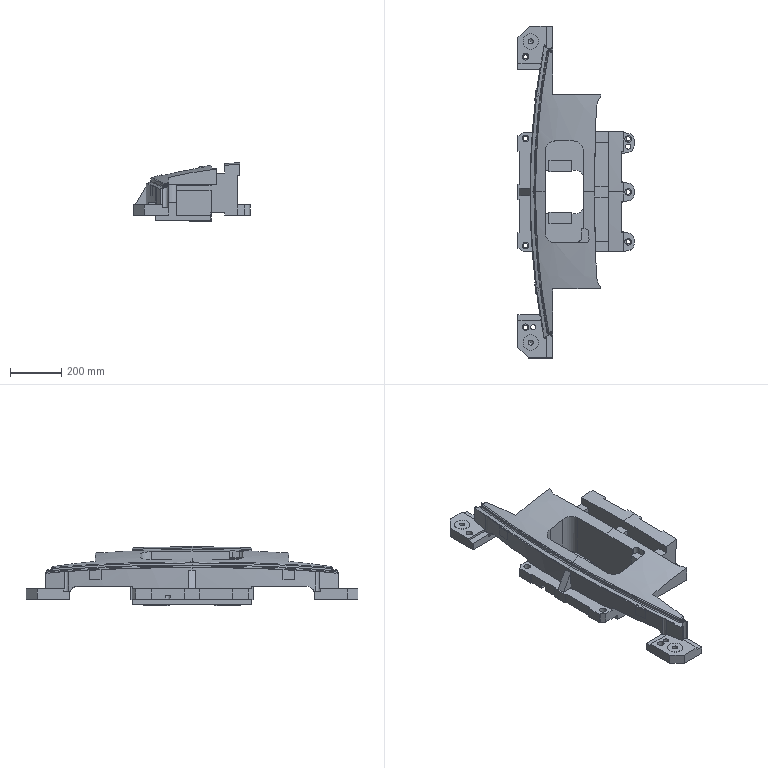Part | NX | features MAIN_BODY 2 | 1 solid | 307 faces | box 455 x 1301 x 231.331 mm | volume 27538350 mm3 | plane 166 | spline 92 | cylinder 47 | cone 2 | commonest cylinder face diameters 17 x7 26 x7 60 x7 20 x6 50 x6 24 x4